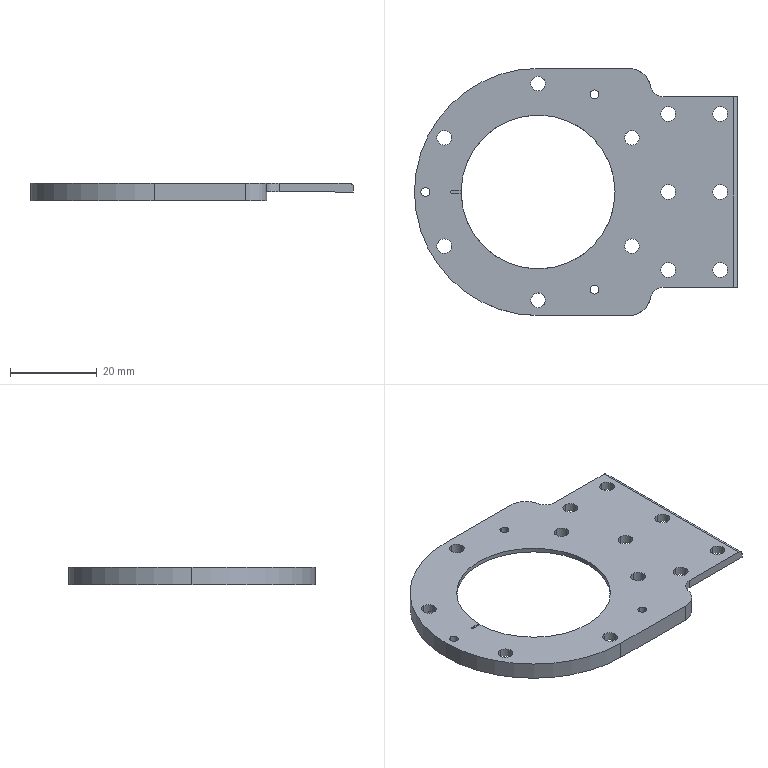NC program | NX | posted with a generic post | part box 74.5 x 57 x 4 mm
Lines 1 to 1524 of 3557:
N10 G17 G21 G94 G90
(FLOOR_WALL , TOOL : D80)
N12 T19 M6
N14 G54
N16 G17 G0 G90 X-82.25 Y0. S5000 M3
N18 G43 Z30. H19
N20 Z3.
N22 G94 G1 Z0. F1200.
N24 X-79.25
N26 X79.25
N28 X82.25
N30 Z3.
N32 G0 Z30.
N34 M5
(SPOT_DRILLING , TOOL : D6A45)
N36 T01 M6
N38 G54
N40 G17 G0 G90 X-8.75 Y-25. S9500 M3
N42 G43 Z30. H1
N44 G94 G82 G98 Z-1. F250. P200 R3.
N46 X4.25 Y-22.517
N48 X12.901 Y-12.5
N50 X21.25 Y-18.
N52 X33.25
N54 Y0.
N56 X21.25
N58 X33.25 Y18.
N60 X21.25
N62 X12.901 Y12.5
N64 X4.25 Y22.517
N66 X-8.75 Y25.
N68 X-30.401 Y12.5
N70 X-34.75 Y0.
N72 X-30.401 Y-12.5
N74 G80
N76 G0 X-30.401 Y-12.5 Z30.
N78 M5
(SPOT_DRILLING_COPY , TOOL : 2.1ZT)
N80 T17 M6
N82 G54
N84 G17 G0 G90 X4.25 Y22.517 S2500 M3
N86 G43 Z30. H17
N88 G94 G83 G98 Z-4.601 F120. Q2. R3.
N90 Y-22.517
N92 X-34.75 Y0.
N94 G80
N96 G0 X-34.75 Y0. Z30.
N98 M5
(SPOT_DRILLING_COPY_COPY , TOOL : 3.4ZT)
N100 T07 M6
N102 G54
N104 G17 G0 G90 X-8.75 Y-25. S2500 M3
N106 G43 Z30. H7
N108 G94 G83 G98 Z-5.021 F120. Q2. R3.
N110 X-30.401 Y-12.5
N112 Y12.5
N114 X-8.75 Y25.
N116 X12.901 Y12.5
N118 X21.25 Y18. Z-3.021
N120 X33.25
N122 Y0.
N124 X21.25
N126 X12.901 Y-12.5 Z-5.021
N128 X21.25 Y-18. Z-3.021
N130 X33.25
N132 G80
N134 G0 X33.25 Y-18. Z30.
N136 M5
(ZLEVEL_PROFILE , TOOL : D10)
N138 T15 M6
N140 G54
N142 G17 G0 G90 X3.196 Y33.6 S9500 M3
N144 G43 Z30. H15
N146 Z1.5
N148 G94 G1 X13.029 Z0.985 F1000.
N150 X15.122 Y33.214 Z0.873
N152 X17.088 Y32.4 Z0.762
N154 X18.841 Y31.193 Z0.65
N156 X20.303 Y29.646 Z0.539
N158 X21.409 Y27.828 Z0.427
N160 X21.687 Y27.1 Z0.386
N162 X37.239 Z-0.429
N164 X37.793 Z-0.458
N166 X39.138 Y26.766 Z-0.531
N168 X40.344 Y26.084 Z-0.603
N170 X41.323 Y25.105 Z-0.676
N172 X42.005 Y23.899 Z-0.748
N174 X42.34 Y22.554 Z-0.821
N176 Y22. Z-0.85
N178 Y-22. F3500.
N180 G2 X37.239 Y-27.1 R5.1
N182 G1 X21.687
N184 G2 X12.25 Y-33.6 R10.1
N186 G1 X-8.75
N188 G2 X-42.35 Y0. R33.6
N190 X-8.75 Y33.6 R33.6
N192 G1 X12.25
N194 G2 X21.687 Y27.1 R10.1
N196 G1 X37.239
N198 G2 X42.34 Y22. R5.1
N200 G1 X42.342 Y17.6 Z-0.864
N202 X42.343 Y13.2 Z-0.878
N204 X42.345 Y8.8 Z-0.893
N206 X42.346 Y4.4 Z-0.907
N208 X42.347 Y0. Z-0.921
N210 X42.348 Y-4.4 Z-0.935
N212 X42.349 Y-8.8 Z-0.95
N214 Y-13.2 Z-0.964
N216 X42.35 Y-17.6 Z-0.978
N218 Y-22. Z-0.992
N220 X42.325 Y-22.501 Z-0.994
N222 X42.251 Y-22.997 Z-0.995
N224 X42.129 Y-23.483 Z-0.997
N226 X41.96 Y-23.955 Z-0.999
N228 X41.745 Y-24.409 Z-1.
N230 X41.487 Y-24.838 Z-1.002
N232 X41.188 Y-25.241 Z-1.004
N234 X40.851 Y-25.612 Z-1.005
N236 X40.479 Y-25.948 Z-1.007
N238 X40.076 Y-26.246 Z-1.008
N240 X39.646 Y-26.502 Z-1.01
N242 X39.192 Y-26.716 Z-1.012
N244 X38.72 Y-26.883 Z-1.013
N246 X38.234 Y-27.004 Z-1.015
N248 X37.745 Y-27.076 Z-1.016
N250 X37.25 Y-27.1 Z-1.018
N252 X21.687 Z-1.068
N254 X21.385 Y-27.809 Z-1.071
N256 X21.039 Y-28.477 Z-1.073
N258 X20.639 Y-29.125 Z-1.076
N260 X20.191 Y-29.741 Z-1.078
N262 X19.699 Y-30.321 Z-1.081
N264 X19.164 Y-30.863 Z-1.083
N266 X18.59 Y-31.363 Z-1.086
N268 X17.979 Y-31.818 Z-1.088
N270 X17.336 Y-32.226 Z-1.09
N272 X16.665 Y-32.584 Z-1.093
N274 X15.968 Y-32.891 Z-1.095
N276 X15.25 Y-33.144 Z-1.098
N278 X14.515 Y-33.343 Z-1.1
N280 X13.767 Y-33.485 Z-1.103
N282 X13.011 Y-33.571 Z-1.105
N284 X12.25 Y-33.6 Z-1.108
N286 X-8.75 Z-1.176
N288 X-10.139 Y-33.571 Z-1.18
N290 X-11.526 Y-33.485 Z-1.185
N292 X-12.908 Y-33.342 Z-1.189
N294 X-14.283 Y-33.141 Z-1.194
N296 X-15.648 Y-32.884 Z-1.198
N298 X-17.002 Y-32.571 Z-1.202
N300 X-18.342 Y-32.202 Z-1.207
N302 X-19.665 Y-31.778 Z-1.211
N304 X-20.969 Y-31.299 Z-1.216
N306 X-22.253 Y-30.767 Z-1.22
N308 X-23.513 Y-30.183 Z-1.225
N310 X-24.749 Y-29.547 Z-1.229
N312 X-25.956 Y-28.86 Z-1.234
N314 X-27.135 Y-28.124 Z-1.238
N316 X-28.282 Y-27.34 Z-1.243
N318 X-29.396 Y-26.509 Z-1.247
N320 X-30.474 Y-25.633 Z-1.252
N322 X-31.515 Y-24.713 Z-1.256
N324 X-32.517 Y-23.75 Z-1.261
N326 X-33.479 Y-22.747 Z-1.265
N328 X-34.398 Y-21.705 Z-1.27
N330 X-35.274 Y-20.627 Z-1.274
N332 X-36.104 Y-19.512 Z-1.279
N334 X-36.887 Y-18.365 Z-1.283
N336 X-37.622 Y-17.186 Z-1.288
N338 X-38.308 Y-15.977 Z-1.292
N340 X-38.943 Y-14.742 Z-1.297
N342 X-39.527 Y-13.481 Z-1.301
N344 X-40.058 Y-12.197 Z-1.306
N346 X-40.536 Y-10.892 Z-1.31
N348 X-40.959 Y-9.568 Z-1.315
N350 X-41.327 Y-8.229 Z-1.319
N352 X-41.639 Y-6.875 Z-1.324
N354 X-41.895 Y-5.509 Z-1.328
N356 X-42.095 Y-4.134 Z-1.333
N358 X-42.237 Y-2.752 Z-1.337
N360 X-42.322 Y-1.365 Z-1.342
N362 X-42.35 Y0.024 Z-1.346
N364 X-42.32 Y1.412 Z-1.351
N366 X-42.233 Y2.797 Z-1.355
N368 X-42.089 Y4.178 Z-1.36
N370 X-41.888 Y5.552 Z-1.364
N372 X-41.631 Y6.916 Z-1.369
N374 X-41.317 Y8.268 Z-1.373
N376 X-40.948 Y9.606 Z-1.378
N378 X-40.523 Y10.928 Z-1.382
N380 X-40.045 Y12.231 Z-1.387
N382 X-39.513 Y13.513 Z-1.391
N384 X-38.928 Y14.772 Z-1.396
N386 X-38.292 Y16.006 Z-1.4
N388 X-37.606 Y17.213 Z-1.404
N390 X-36.87 Y18.39 Z-1.409
N392 X-36.087 Y19.536 Z-1.413
N394 X-35.257 Y20.649 Z-1.418
N396 X-34.381 Y21.726 Z-1.422
N398 X-33.462 Y22.766 Z-1.427
N400 X-32.5 Y23.767 Z-1.431
N402 X-31.498 Y24.728 Z-1.436
N404 X-30.457 Y25.647 Z-1.44
N406 X-29.38 Y26.521 Z-1.445
N408 X-28.266 Y27.351 Z-1.449
N410 X-27.12 Y28.134 Z-1.454
N412 X-25.942 Y28.868 Z-1.458
N414 X-24.735 Y29.554 Z-1.463
N416 X-23.501 Y30.189 Z-1.467
N418 X-22.241 Y30.773 Z-1.472
N420 X-20.959 Y31.304 Z-1.476
N422 X-19.655 Y31.781 Z-1.481
N424 X-18.333 Y32.204 Z-1.485
N426 X-16.995 Y32.573 Z-1.49
N428 X-15.642 Y32.886 Z-1.494
N430 X-14.278 Y33.142 Z-1.499
N432 X-12.904 Y33.342 Z-1.503
N434 X-11.523 Y33.485 Z-1.508
N436 X-10.138 Y33.571 Z-1.512
N438 X-8.75 Y33.6 Z-1.517
N440 X12.25 Z-1.585
N442 X13.011 Y33.571 Z-1.587
N444 X13.767 Y33.485 Z-1.589
N446 X14.515 Y33.343 Z-1.592
N448 X15.25 Y33.144 Z-1.594
N450 X15.968 Y32.891 Z-1.597
N452 X16.665 Y32.584 Z-1.599
N454 X17.336 Y32.226 Z-1.602
N456 X17.979 Y31.818 Z-1.604
N458 X18.59 Y31.363 Z-1.607
N460 X19.164 Y30.863 Z-1.609
N462 X19.699 Y30.321 Z-1.612
N464 X20.191 Y29.741 Z-1.614
N466 X20.639 Y29.125 Z-1.616
N468 X21.039 Y28.477 Z-1.619
N470 X21.385 Y27.809 Z-1.621
N472 X21.687 Y27.1 Z-1.624
N474 X37.25 Z-1.674
N476 X37.745 Y27.076 Z-1.676
N478 X38.234 Y27.004 Z-1.677
N480 X38.72 Y26.883 Z-1.679
N482 X39.192 Y26.716 Z-1.681
N484 X39.646 Y26.502 Z-1.682
N486 X40.076 Y26.246 Z-1.684
N488 X40.479 Y25.948 Z-1.685
N490 X40.851 Y25.612 Z-1.687
N492 X41.188 Y25.241 Z-1.689
N494 X41.487 Y24.838 Z-1.69
N496 X41.745 Y24.409 Z-1.692
N498 X41.96 Y23.956 Z-1.694
N500 X42.129 Y23.483 Z-1.695
N502 X42.252 Y22.997 Z-1.697
N504 X42.325 Y22.501 Z-1.698
N506 X42.35 Y22. Z-1.7
N508 Y-22. Z-1.842
N510 X42.325 Y-22.5 Z-1.844
N512 X42.252 Y-22.995 Z-1.845
N514 X42.13 Y-23.48 Z-1.847
N516 X41.962 Y-23.952 Z-1.849
N518 X41.748 Y-24.404 Z-1.85
N520 X41.49 Y-24.833 Z-1.852
N522 X41.192 Y-25.235 Z-1.854
N524 X40.856 Y-25.606 Z-1.855
N526 X40.485 Y-25.942 Z-1.857
N528 X40.083 Y-26.24 Z-1.858
N530 X39.654 Y-26.498 Z-1.86
N532 X39.202 Y-26.712 Z-1.862
N534 X38.73 Y-26.88 Z-1.863
N536 X38.245 Y-27.002 Z-1.865
N538 X37.75 Y-27.075 Z-1.866
N540 X37.25 Y-27.1 Z-1.868
N542 X21.687 Z-1.918
N544 X21.385 Y-27.809 Z-1.921
N546 X21.039 Y-28.477 Z-1.923
N548 X20.639 Y-29.125 Z-1.926
N550 X20.191 Y-29.741 Z-1.928
N552 X19.699 Y-30.321 Z-1.931
N554 X19.164 Y-30.863 Z-1.933
N556 X18.59 Y-31.363 Z-1.936
N558 X17.979 Y-31.818 Z-1.938
N560 X17.336 Y-32.226 Z-1.94
N562 X16.665 Y-32.584 Z-1.943
N564 X15.968 Y-32.891 Z-1.945
N566 X15.25 Y-33.144 Z-1.948
N568 X14.515 Y-33.343 Z-1.95
N570 X13.767 Y-33.485 Z-1.953
N572 X13.011 Y-33.571 Z-1.955
N574 X12.25 Y-33.6 Z-1.958
N576 X-8.75 Z-2.026
N578 X-10.139 Y-33.571 Z-2.03
N580 X-11.526 Y-33.485 Z-2.035
N582 X-12.908 Y-33.342 Z-2.039
N584 X-14.283 Y-33.141 Z-2.044
N586 X-15.648 Y-32.884 Z-2.048
N588 X-17.002 Y-32.571 Z-2.053
N590 X-18.342 Y-32.202 Z-2.057
N592 X-19.665 Y-31.778 Z-2.061
N594 X-20.969 Y-31.299 Z-2.066
N596 X-22.253 Y-30.767 Z-2.07
N598 X-23.513 Y-30.183 Z-2.075
N600 X-24.749 Y-29.547 Z-2.079
N602 X-25.956 Y-28.86 Z-2.084
N604 X-27.135 Y-28.124 Z-2.088
N606 X-28.282 Y-27.34 Z-2.093
N608 X-29.396 Y-26.509 Z-2.097
N610 X-30.474 Y-25.633 Z-2.102
N612 X-31.515 Y-24.713 Z-2.106
N614 X-32.517 Y-23.75 Z-2.111
N616 X-33.479 Y-22.747 Z-2.115
N618 X-34.398 Y-21.705 Z-2.12
N620 X-35.274 Y-20.627 Z-2.124
N622 X-36.104 Y-19.512 Z-2.129
N624 X-36.887 Y-18.365 Z-2.133
N626 X-37.622 Y-17.186 Z-2.138
N628 X-38.308 Y-15.977 Z-2.142
N630 X-38.943 Y-14.742 Z-2.147
N632 X-39.527 Y-13.481 Z-2.151
N634 X-40.058 Y-12.197 Z-2.156
N636 X-40.536 Y-10.892 Z-2.16
N638 X-40.959 Y-9.568 Z-2.165
N640 X-41.327 Y-8.229 Z-2.169
N642 X-41.639 Y-6.875 Z-2.174
N644 X-41.895 Y-5.509 Z-2.178
N646 X-42.095 Y-4.134 Z-2.183
N648 X-42.237 Y-2.752 Z-2.187
N650 X-42.322 Y-1.365 Z-2.192
N652 X-42.35 Y0.024 Z-2.196
N654 X-42.32 Y1.412 Z-2.201
N656 X-42.233 Y2.797 Z-2.205
N658 X-42.089 Y4.178 Z-2.21
N660 X-41.888 Y5.552 Z-2.214
N662 X-41.631 Y6.916 Z-2.219
N664 X-41.317 Y8.268 Z-2.223
N666 X-40.948 Y9.606 Z-2.228
N668 X-40.523 Y10.928 Z-2.232
N670 X-40.045 Y12.231 Z-2.237
N672 X-39.513 Y13.513 Z-2.241
N674 X-38.928 Y14.772 Z-2.246
N676 X-38.292 Y16.006 Z-2.25
N678 X-37.606 Y17.213 Z-2.254
N680 X-36.87 Y18.39 Z-2.259
N682 X-36.087 Y19.536 Z-2.263
N684 X-35.257 Y20.649 Z-2.268
N686 X-34.381 Y21.726 Z-2.272
N688 X-33.462 Y22.766 Z-2.277
N690 X-32.5 Y23.767 Z-2.281
N692 X-31.498 Y24.728 Z-2.286
N694 X-30.457 Y25.647 Z-2.29
N696 X-29.38 Y26.521 Z-2.295
N698 X-28.266 Y27.351 Z-2.299
N700 X-27.12 Y28.134 Z-2.304
N702 X-25.942 Y28.868 Z-2.308
N704 X-24.735 Y29.554 Z-2.313
N706 X-23.501 Y30.189 Z-2.317
N708 X-22.241 Y30.773 Z-2.322
N710 X-20.959 Y31.304 Z-2.326
N712 X-19.655 Y31.781 Z-2.331
N714 X-18.333 Y32.204 Z-2.335
N716 X-16.995 Y32.573 Z-2.34
N718 X-15.642 Y32.886 Z-2.344
N720 X-14.278 Y33.142 Z-2.349
N722 X-12.904 Y33.342 Z-2.353
N724 X-11.523 Y33.485 Z-2.358
N726 X-10.138 Y33.571 Z-2.362
N728 X-8.75 Y33.6 Z-2.367
N730 X12.25 Z-2.435
N732 X13.011 Y33.571 Z-2.437
N734 X13.767 Y33.485 Z-2.439
N736 X14.515 Y33.343 Z-2.442
N738 X15.25 Y33.144 Z-2.444
N740 X15.968 Y32.891 Z-2.447
N742 X16.665 Y32.584 Z-2.449
N744 X17.336 Y32.226 Z-2.452
N746 X17.979 Y31.818 Z-2.454
N748 X18.59 Y31.363 Z-2.457
N750 X19.164 Y30.863 Z-2.459
N752 X19.699 Y30.321 Z-2.462
N754 X20.191 Y29.741 Z-2.464
N756 X20.639 Y29.125 Z-2.466
N758 X21.039 Y28.477 Z-2.469
N760 X21.385 Y27.809 Z-2.471
N762 X21.687 Y27.1 Z-2.474
N764 X37.25 Z-2.524
N766 X37.75 Y27.075 Z-2.526
N768 X38.245 Y27.002 Z-2.527
N770 X38.73 Y26.88 Z-2.529
N772 X39.202 Y26.712 Z-2.531
N774 X39.654 Y26.498 Z-2.532
N776 X40.083 Y26.241 Z-2.534
N778 X40.485 Y25.942 Z-2.535
N780 X40.856 Y25.606 Z-2.537
N782 X41.192 Y25.235 Z-2.539
N784 X41.49 Y24.833 Z-2.54
N786 X41.748 Y24.404 Z-2.542
N788 X41.962 Y23.952 Z-2.544
N790 X42.13 Y23.48 Z-2.545
N792 X42.252 Y22.995 Z-2.547
N794 X42.325 Y22.5 Z-2.548
N796 X42.35 Y22. Z-2.55
N798 Y-22. Z-2.692
N800 X42.325 Y-22.5 Z-2.694
N802 X42.252 Y-22.995 Z-2.695
N804 X42.13 Y-23.48 Z-2.697
N806 X41.962 Y-23.952 Z-2.699
N808 X41.748 Y-24.404 Z-2.7
N810 X41.49 Y-24.833 Z-2.702
N812 X41.192 Y-25.235 Z-2.704
N814 X40.856 Y-25.606 Z-2.705
N816 X40.485 Y-25.942 Z-2.707
N818 X40.083 Y-26.24 Z-2.708
N820 X39.654 Y-26.498 Z-2.71
N822 X39.202 Y-26.712 Z-2.712
N824 X38.73 Y-26.88 Z-2.713
N826 X38.245 Y-27.002 Z-2.715
N828 X37.75 Y-27.075 Z-2.716
N830 X37.25 Y-27.1 Z-2.718
N832 X21.687 Z-2.768
N834 X21.385 Y-27.809 Z-2.771
N836 X21.039 Y-28.477 Z-2.773
N838 X20.639 Y-29.125 Z-2.776
N840 X20.191 Y-29.741 Z-2.778
N842 X19.699 Y-30.321 Z-2.781
N844 X19.164 Y-30.863 Z-2.783
N846 X18.59 Y-31.363 Z-2.786
N848 X17.979 Y-31.818 Z-2.788
N850 X17.336 Y-32.226 Z-2.79
N852 X16.665 Y-32.584 Z-2.793
N854 X15.968 Y-32.891 Z-2.795
N856 X15.25 Y-33.144 Z-2.798
N858 X14.515 Y-33.343 Z-2.8
N860 X13.767 Y-33.485 Z-2.803
N862 X13.011 Y-33.571 Z-2.805
N864 X12.25 Y-33.6 Z-2.808
N866 X-8.75 Z-2.876
N868 X-10.139 Y-33.571 Z-2.88
N870 X-11.526 Y-33.485 Z-2.885
N872 X-12.908 Y-33.342 Z-2.889
N874 X-14.283 Y-33.141 Z-2.894
N876 X-15.648 Y-32.884 Z-2.898
N878 X-17.002 Y-32.571 Z-2.903
N880 X-18.342 Y-32.202 Z-2.907
N882 X-19.665 Y-31.778 Z-2.911
N884 X-20.969 Y-31.299 Z-2.916
N886 X-22.253 Y-30.767 Z-2.92
N888 X-23.513 Y-30.183 Z-2.925
N890 X-24.749 Y-29.547 Z-2.929
N892 X-25.956 Y-28.86 Z-2.934
N894 X-27.135 Y-28.124 Z-2.938
N896 X-28.282 Y-27.34 Z-2.943
N898 X-29.396 Y-26.509 Z-2.947
N900 X-30.474 Y-25.633 Z-2.952
N902 X-31.515 Y-24.713 Z-2.956
N904 X-32.517 Y-23.75 Z-2.961
N906 X-33.479 Y-22.747 Z-2.965
N908 X-34.398 Y-21.705 Z-2.97
N910 X-35.274 Y-20.627 Z-2.974
N912 X-36.104 Y-19.512 Z-2.979
N914 X-36.887 Y-18.365 Z-2.983
N916 X-37.622 Y-17.186 Z-2.988
N918 X-38.308 Y-15.977 Z-2.992
N920 X-38.943 Y-14.742 Z-2.997
N922 X-39.527 Y-13.481 Z-3.001
N924 X-40.058 Y-12.197 Z-3.006
N926 X-40.536 Y-10.892 Z-3.01
N928 X-40.959 Y-9.568 Z-3.015
N930 X-41.327 Y-8.229 Z-3.019
N932 X-41.639 Y-6.875 Z-3.024
N934 X-41.895 Y-5.509 Z-3.028
N936 X-42.095 Y-4.134 Z-3.033
N938 X-42.237 Y-2.752 Z-3.037
N940 X-42.322 Y-1.365 Z-3.042
N942 X-42.35 Y0.024 Z-3.046
N944 X-42.32 Y1.412 Z-3.051
N946 X-42.233 Y2.797 Z-3.055
N948 X-42.089 Y4.178 Z-3.06
N950 X-41.888 Y5.552 Z-3.064
N952 X-41.631 Y6.916 Z-3.069
N954 X-41.317 Y8.268 Z-3.073
N956 X-40.948 Y9.606 Z-3.078
N958 X-40.523 Y10.928 Z-3.082
N960 X-40.045 Y12.231 Z-3.087
N962 X-39.513 Y13.513 Z-3.091
N964 X-38.928 Y14.772 Z-3.096
N966 X-38.292 Y16.006 Z-3.1
N968 X-37.606 Y17.213 Z-3.104
N970 X-36.87 Y18.39 Z-3.109
N972 X-36.087 Y19.536 Z-3.113
N974 X-35.257 Y20.649 Z-3.118
N976 X-34.381 Y21.726 Z-3.122
N978 X-33.462 Y22.766 Z-3.127
N980 X-32.5 Y23.767 Z-3.131
N982 X-31.498 Y24.728 Z-3.136
N984 X-30.457 Y25.647 Z-3.14
N986 X-29.38 Y26.521 Z-3.145
N988 X-28.266 Y27.351 Z-3.149
N990 X-27.12 Y28.134 Z-3.154
N992 X-25.942 Y28.868 Z-3.158
N994 X-24.735 Y29.554 Z-3.163
N996 X-23.501 Y30.189 Z-3.167
N998 X-22.241 Y30.773 Z-3.172
N1000 X-20.959 Y31.304 Z-3.176
N1002 X-19.655 Y31.781 Z-3.181
N1004 X-18.333 Y32.204 Z-3.185
N1006 X-16.995 Y32.573 Z-3.19
N1008 X-15.642 Y32.886 Z-3.194
N1010 X-14.278 Y33.142 Z-3.199
N1012 X-12.904 Y33.342 Z-3.203
N1014 X-11.523 Y33.485 Z-3.208
N1016 X-10.138 Y33.571 Z-3.212
N1018 X-8.75 Y33.6 Z-3.217
N1020 X12.25 Z-3.285
N1022 X13.011 Y33.571 Z-3.287
N1024 X13.767 Y33.485 Z-3.289
N1026 X14.515 Y33.343 Z-3.292
N1028 X15.25 Y33.144 Z-3.294
N1030 X15.968 Y32.891 Z-3.297
N1032 X16.665 Y32.584 Z-3.299
N1034 X17.336 Y32.226 Z-3.302
N1036 X17.979 Y31.818 Z-3.304
N1038 X18.59 Y31.363 Z-3.307
N1040 X19.164 Y30.863 Z-3.309
N1042 X19.699 Y30.321 Z-3.312
N1044 X20.191 Y29.741 Z-3.314
N1046 X20.639 Y29.125 Z-3.316
N1048 X21.039 Y28.477 Z-3.319
N1050 X21.385 Y27.809 Z-3.321
N1052 X21.687 Y27.1 Z-3.324
N1054 X37.25 Z-3.374
N1056 X37.75 Y27.075 Z-3.376
N1058 X38.245 Y27.002 Z-3.377
N1060 X38.73 Y26.88 Z-3.379
N1062 X39.202 Y26.712 Z-3.381
N1064 X39.654 Y26.498 Z-3.382
N1066 X40.083 Y26.241 Z-3.384
N1068 X40.485 Y25.942 Z-3.385
N1070 X40.856 Y25.606 Z-3.387
N1072 X41.192 Y25.235 Z-3.389
N1074 X41.49 Y24.833 Z-3.39
N1076 X41.748 Y24.404 Z-3.392
N1078 X41.962 Y23.952 Z-3.394
N1080 X42.13 Y23.48 Z-3.395
N1082 X42.252 Y22.995 Z-3.397
N1084 X42.325 Y22.5 Z-3.398
N1086 X42.35 Y22. Z-3.4
N1088 Y-22.
N1090 G2 X37.25 Y-27.1 R5.1
N1092 G1 X21.687
N1094 G2 X12.25 Y-33.6 R10.1
N1096 G1 X-8.75
N1098 G2 X-42.35 Y0. R33.6
N1100 X-8.75 Y33.6 R33.6
N1102 G1 X12.25
N1104 G2 X21.687 Y27.1 R10.1
N1106 G1 X37.25
N1108 G2 X42.35 Y22. R5.1
N1110 G1 Z-1.9
N1112 G0 Z30.
(PLANAR_MILL_3 , TOOL : D10)
N1114 X-14.863 Y-0.634
N1116 Z1.5
N1118 G1 X-14.784 Y-1.24 Z1.468 F1000.
N1120 X-14.54 Y-2.103 Z1.421
N1122 X-14.173 Y-2.921 Z1.374
N1124 X-13.692 Y-3.677 Z1.327
N1126 X-13.106 Y-4.356 Z1.28
N1128 X-12.427 Y-4.942 Z1.233
N1130 X-11.671 Y-5.423 Z1.186
N1132 X-10.853 Y-5.79 Z1.139
N1134 X-9.99 Y-6.034 Z1.092
N1136 X-9.101 Y-6.15 Z1.045
N1138 X-8.399 Z1.008
N1140 X-7.51 Y-6.034 Z0.961
N1142 X-6.647 Y-5.79 Z0.914
N1144 X-5.829 Y-5.423 Z0.867
N1146 X-5.073 Y-4.942 Z0.82
N1148 X-4.394 Y-4.356 Z0.773
N1150 X-3.808 Y-3.677 Z0.726
N1152 X-3.327 Y-2.921 Z0.679
N1154 X-2.96 Y-2.103 Z0.632
N1156 X-2.716 Y-1.24 Z0.585
N1158 X-2.6 Y-0.351 Z0.538
N1160 Y0.351 Z0.502
N1162 X-2.716 Y1.24 Z0.455
N1164 X-2.96 Y2.103 Z0.408
N1166 X-3.327 Y2.921 Z0.361
N1168 X-3.808 Y3.677 Z0.314
N1170 X-4.394 Y4.356 Z0.267
N1172 X-5.073 Y4.942 Z0.22
N1174 X-5.829 Y5.423 Z0.173
N1176 X-6.647 Y5.79 Z0.126
N1178 X-7.51 Y6.034 Z0.079
N1180 X-8.399 Y6.15 Z0.032
N1182 X-9.101 Z-0.005
N1184 X-9.99 Y6.034 Z-0.052
N1186 X-10.853 Y5.79 Z-0.099
N1188 X-11.671 Y5.423 Z-0.146
N1190 X-12.427 Y4.942 Z-0.193
N1192 X-13.106 Y4.356 Z-0.24
N1194 X-13.692 Y3.677 Z-0.287
N1196 X-14.173 Y2.921 Z-0.334
N1198 X-14.54 Y2.103 Z-0.381
N1200 X-14.784 Y1.24 Z-0.428
N1202 X-14.9 Y0.351 Z-0.475
N1204 Y-0.351 Z-0.512
N1206 X-14.784 Y-1.24 Z-0.559
N1208 X-14.54 Y-2.103 Z-0.606
N1210 X-14.173 Y-2.921 Z-0.653
N1212 X-13.692 Y-3.677 Z-0.7
N1214 X-13.106 Y-4.356 Z-0.747
N1216 X-12.427 Y-4.942 Z-0.794
N1218 X-11.671 Y-5.423 Z-0.841
N1220 X-10.853 Y-5.79 Z-0.888
N1222 X-9.99 Y-6.034 Z-0.935
N1224 X-9.101 Y-6.15 Z-0.982
N1226 X-8.75 Z-1.
N1228 Y-1.65
N1230 G3 X-7.1 Y0. R1.65 F3500.
N1232 X-8.75 Y-1.65 R-1.65
N1234 G1 Y-6.15
N1236 G3 X-2.6 Y0. R6.15
N1238 X-8.75 Y-6.15 R-6.15
N1240 G1 Y-12.65
N1242 G3 X3.9 Y0. R12.65
N1244 X-8.75 Y-12.65 R-12.65
N1246 G1 Z0.5
N1248 G0 X-14.863 Y-0.634
N1250 G1 X-14.784 Y-1.24 Z0.468 F1000.
N1252 X-14.54 Y-2.103 Z0.421
N1254 X-14.173 Y-2.921 Z0.374
N1256 X-13.692 Y-3.677 Z0.327
N1258 X-13.106 Y-4.356 Z0.28
N1260 X-12.427 Y-4.942 Z0.233
N1262 X-11.671 Y-5.423 Z0.186
N1264 X-10.853 Y-5.79 Z0.139
N1266 X-9.99 Y-6.034 Z0.092
N1268 X-9.101 Y-6.15 Z0.045
N1270 X-8.399 Z0.008
N1272 X-7.51 Y-6.034 Z-0.039
N1274 X-6.647 Y-5.79 Z-0.086
N1276 X-5.829 Y-5.423 Z-0.133
N1278 X-5.073 Y-4.942 Z-0.18
N1280 X-4.394 Y-4.356 Z-0.227
N1282 X-3.808 Y-3.677 Z-0.274
N1284 X-3.327 Y-2.921 Z-0.321
N1286 X-2.96 Y-2.103 Z-0.368
N1288 X-2.716 Y-1.24 Z-0.415
N1290 X-2.6 Y-0.351 Z-0.462
N1292 Y0.351 Z-0.498
N1294 X-2.716 Y1.24 Z-0.545
N1296 X-2.96 Y2.103 Z-0.592
N1298 X-3.327 Y2.921 Z-0.639
N1300 X-3.808 Y3.677 Z-0.686
N1302 X-4.394 Y4.356 Z-0.733
N1304 X-5.073 Y4.942 Z-0.78
N1306 X-5.829 Y5.423 Z-0.827
N1308 X-6.647 Y5.79 Z-0.874
N1310 X-7.51 Y6.034 Z-0.921
N1312 X-8.399 Y6.15 Z-0.968
N1314 X-9.101 Z-1.005
N1316 X-9.99 Y6.034 Z-1.052
N1318 X-10.853 Y5.79 Z-1.099
N1320 X-11.671 Y5.423 Z-1.146
N1322 X-12.427 Y4.942 Z-1.193
N1324 X-13.106 Y4.356 Z-1.24
N1326 X-13.692 Y3.677 Z-1.287
N1328 X-14.173 Y2.921 Z-1.334
N1330 X-14.54 Y2.103 Z-1.381
N1332 X-14.784 Y1.24 Z-1.428
N1334 X-14.9 Y0.351 Z-1.475
N1336 Y-0.351 Z-1.512
N1338 X-14.784 Y-1.24 Z-1.559
N1340 X-14.54 Y-2.103 Z-1.606
N1342 X-14.173 Y-2.921 Z-1.653
N1344 X-13.692 Y-3.677 Z-1.7
N1346 X-13.106 Y-4.356 Z-1.747
N1348 X-12.427 Y-4.942 Z-1.794
N1350 X-11.671 Y-5.423 Z-1.841
N1352 X-10.853 Y-5.79 Z-1.888
N1354 X-9.99 Y-6.034 Z-1.935
N1356 X-9.101 Y-6.15 Z-1.982
N1358 X-8.75 Z-2.
N1360 Y-1.65
N1362 G3 X-7.1 Y0. R1.65 F3500.
N1364 X-8.75 Y-1.65 R-1.65
N1366 G1 Y-6.15
N1368 G3 X-2.6 Y0. R6.15
N1370 X-8.75 Y-6.15 R-6.15
N1372 G1 Y-12.65
N1374 G3 X3.9 Y0. R12.65
N1376 X-8.75 Y-12.65 R-12.65
N1378 G1 Z-0.5
N1380 G0 X-14.863 Y-0.634
N1382 G1 X-14.784 Y-1.24 Z-0.532 F1000.
N1384 X-14.54 Y-2.103 Z-0.579
N1386 X-14.173 Y-2.921 Z-0.626
N1388 X-13.692 Y-3.677 Z-0.673
N1390 X-13.106 Y-4.356 Z-0.72
N1392 X-12.427 Y-4.942 Z-0.767
N1394 X-11.671 Y-5.423 Z-0.814
N1396 X-10.853 Y-5.79 Z-0.861
N1398 X-9.99 Y-6.034 Z-0.908
N1400 X-9.101 Y-6.15 Z-0.955
N1402 X-8.399 Z-0.992
N1404 X-7.51 Y-6.034 Z-1.039
N1406 X-6.647 Y-5.79 Z-1.086
N1408 X-5.829 Y-5.423 Z-1.133
N1410 X-5.073 Y-4.942 Z-1.18
N1412 X-4.394 Y-4.356 Z-1.227
N1414 X-3.808 Y-3.677 Z-1.274
N1416 X-3.327 Y-2.921 Z-1.321
N1418 X-2.96 Y-2.103 Z-1.368
N1420 X-2.716 Y-1.24 Z-1.415
N1422 X-2.6 Y-0.351 Z-1.462
N1424 Y0.351 Z-1.498
N1426 X-2.716 Y1.24 Z-1.545
N1428 X-2.96 Y2.103 Z-1.592
N1430 X-3.327 Y2.921 Z-1.639
N1432 X-3.808 Y3.677 Z-1.686
N1434 X-4.394 Y4.356 Z-1.733
N1436 X-5.073 Y4.942 Z-1.78
N1438 X-5.829 Y5.423 Z-1.827
N1440 X-6.647 Y5.79 Z-1.874
N1442 X-7.51 Y6.034 Z-1.921
N1444 X-8.399 Y6.15 Z-1.968
N1446 X-9.101 Z-2.005
N1448 X-9.99 Y6.034 Z-2.052
N1450 X-10.853 Y5.79 Z-2.099
N1452 X-11.671 Y5.423 Z-2.146
N1454 X-12.427 Y4.942 Z-2.193
N1456 X-13.106 Y4.356 Z-2.24
N1458 X-13.692 Y3.677 Z-2.287
N1460 X-14.173 Y2.921 Z-2.334
N1462 X-14.54 Y2.103 Z-2.381
N1464 X-14.784 Y1.24 Z-2.428
N1466 X-14.9 Y0.351 Z-2.475
N1468 Y-0.351 Z-2.512
N1470 X-14.784 Y-1.24 Z-2.559
N1472 X-14.54 Y-2.103 Z-2.606
N1474 X-14.173 Y-2.921 Z-2.653
N1476 X-13.692 Y-3.677 Z-2.7
N1478 X-13.106 Y-4.356 Z-2.747
N1480 X-12.427 Y-4.942 Z-2.794
N1482 X-11.671 Y-5.423 Z-2.841
N1484 X-10.853 Y-5.79 Z-2.888
N1486 X-9.99 Y-6.034 Z-2.935
N1488 X-9.101 Y-6.15 Z-2.982
N1490 X-8.75 Z-3.
N1492 Y-1.65
N1494 G3 X-7.1 Y0. R1.65 F3500.
N1496 X-8.75 Y-1.65 R-1.65
N1498 G1 Y-6.15
N1500 G3 X-2.6 Y0. R6.15
N1502 X-8.75 Y-6.15 R-6.15
N1504 G1 Y-12.65
N1506 G3 X3.9 Y0. R12.65
N1508 X-8.75 Y-12.65 R-12.65
N1510 G1 Z-1.5
N1512 G0 X-14.863 Y-0.634
N1514 G1 X-14.784 Y-1.24 Z-1.532 F1000.
N1516 X-14.54 Y-2.103 Z-1.579
N1518 X-14.173 Y-2.921 Z-1.626
N1520 X-13.692 Y-3.677 Z-1.673
N1522 X-13.106 Y-4.356 Z-1.72
N1524 X-12.427 Y-4.942 Z-1.767
N1526 X-11.671 Y-5.423 Z-1.814
N1528 X-10.853 Y-5.79 Z-1.861
N1530 X-9.99 Y-6.034 Z-1.908
N1532 X-9.101 Y-6.15 Z-1.955
N1534 X-8.399 Z-1.992
N1536 X-7.51 Y-6.034 Z-2.039
N1538 X-6.647 Y-5.79 Z-2.086
N1540 X-5.829 Y-5.423 Z-2.133
N1542 X-5.073 Y-4.942 Z-2.18
N1544 X-4.394 Y-4.356 Z-2.227
N1546 X-3.808 Y-3.677 Z-2.274
N1548 X-3.327 Y-2.921 Z-2.321
N1550 X-2.96 Y-2.103 Z-2.368
N1552 X-2.716 Y-1.24 Z-2.415
N1554 X-2.6 Y-0.351 Z-2.462
N1556 Y0.351 Z-2.498
N1558 X-2.716 Y1.24 Z-2.545
N1560 X-2.96 Y2.103 Z-2.592
N1562 X-3.327 Y2.921 Z-2.639
N1564 X-3.808 Y3.677 Z-2.686
N1566 X-4.394 Y4.356 Z-2.733
N1568 X-5.073 Y4.942 Z-2.78
N1570 X-5.829 Y5.423 Z-2.827
N1572 X-6.647 Y5.79 Z-2.874
N1574 X-7.51 Y6.034 Z-2.921
N1576 X-8.399 Y6.15 Z-2.968
N1578 X-9.101 Z-3.005
N1580 X-9.99 Y6.034 Z-3.052
N1582 X-10.853 Y5.79 Z-3.099
N1584 X-11.671 Y5.423 Z-3.146
N1586 X-12.427 Y4.942 Z-3.193
N1588 X-13.106 Y4.356 Z-3.24
N1590 X-13.692 Y3.677 Z-3.287
N1592 X-14.173 Y2.921 Z-3.334
N1594 X-14.54 Y2.103 Z-3.381
N1596 X-14.784 Y1.24 Z-3.428
N1598 X-14.9 Y0.351 Z-3.475
N1600 Y-0.351 Z-3.512
N1602 X-14.784 Y-1.24 Z-3.559
N1604 X-14.54 Y-2.103 Z-3.606
N1606 X-14.173 Y-2.921 Z-3.653
N1608 X-13.692 Y-3.677 Z-3.7
N1610 X-13.106 Y-4.356 Z-3.747
N1612 X-12.427 Y-4.942 Z-3.794
N1614 X-11.671 Y-5.423 Z-3.841
N1616 X-10.853 Y-5.79 Z-3.888
N1618 X-9.99 Y-6.034 Z-3.935
N1620 X-9.101 Y-6.15 Z-3.982
N1622 X-8.75 Z-4.
N1624 Y-1.65
N1626 G3 X-7.1 Y0. R1.65 F3500.
N1628 X-8.75 Y-1.65 R-1.65
N1630 G1 Y-6.15
N1632 G3 X-2.6 Y0. R6.15
N1634 X-8.75 Y-6.15 R-6.15
N1636 G1 Y-12.65
N1638 G3 X3.9 Y0. R12.65
N1640 X-8.75 Y-12.65 R-12.65
N1642 G1 Z-2.5
N1644 G0 Z30.
N1646 M5
(ZLEVEL_PROFILE_COPY_1 , TOOL : D3)
N1648 T16 M6
N1650 G54
N1652 G17 G0 G90 X18.613 Y26.651 S9500 M3
N1654 G43 Z30. H16
N1656 Z1.214
N1658 G94 G1 Z-0.286 F1000.
N1660 X18.307 Y26.257
N1662 G3 X18.267 Y25.959 R0.3
N1664 G2 X18.635 Y24.719 R6.5 F1200.
N1666 G3 X20.108 Y23.5 R1.5
N1668 G1 X21.743
N1670 G3 X22.003 Y23.65 R0.3
N1672 G1 X22.262 Y24.1
N1674 Z1.214
N1676 G0 X18.613 Y26.651 Z0.929
N1678 G1 Z-0.571 F1000.
N1680 X18.307 Y26.257
N1682 G3 X18.267 Y25.959 R0.3
N1684 G2 X18.635 Y24.719 R6.5 F1200.
N1686 G3 X20.108 Y23.5 R1.5
N1688 G1 X21.743
N1690 G3 X22.003 Y23.65 R0.3
N1692 G1 X22.262 Y24.1
N1694 Z0.929
N1696 G0 X18.613 Y26.651 Z0.643
N1698 G1 Z-0.857 F1000.
N1700 X18.307 Y26.257
N1702 G3 X18.267 Y25.959 R0.3
N1704 G2 X18.635 Y24.719 R6.5 F1200.
N1706 G3 X20.108 Y23.5 R1.5
N1708 G1 X21.743
N1710 G3 X22.003 Y23.65 R0.3
N1712 G1 X22.262 Y24.1
N1714 Z0.643
N1716 G0 X18.613 Y26.651 Z0.357
N1718 G1 Z-1.143 F1000.
N1720 X18.307 Y26.257
N1722 G3 X18.267 Y25.959 R0.3
N1724 G2 X18.635 Y24.719 R6.5 F1200.
N1726 G3 X20.108 Y23.5 R1.5
N1728 G1 X21.743
N1730 G3 X22.003 Y23.65 R0.3
N1732 G1 X22.262 Y24.1
N1734 Z0.357
N1736 G0 X18.613 Y26.651 Z0.071
N1738 G1 Z-1.429 F1000.
N1740 X18.307 Y26.257
N1742 G3 X18.267 Y25.959 R0.3
N1744 G2 X18.635 Y24.719 R6.5 F1200.
N1746 G3 X20.108 Y23.5 R1.5
N1748 G1 X21.743
N1750 G3 X22.003 Y23.65 R0.3
N1752 G1 X22.262 Y24.1
N1754 Z0.071
N1756 G0 X18.613 Y26.651 Z-0.214
N1758 G1 Z-1.714 F1000.
N1760 X18.307 Y26.257
N1762 G3 X18.267 Y25.959 R0.3
N1764 G2 X18.635 Y24.719 R6.5 F1200.
N1766 G3 X20.108 Y23.5 R1.5
N1768 G1 X21.743
N1770 G3 X22.003 Y23.65 R0.3
N1772 G1 X22.262 Y24.1
N1774 Z-0.214
N1776 G0 X18.613 Y26.651 Z-0.5
N1778 G1 Z-2. F1000.
N1780 X18.307 Y26.257
N1782 G3 X18.267 Y25.959 R0.3
N1784 G2 X18.635 Y24.719 R6.5 F1200.
N1786 G3 X20.108 Y23.5 R1.5
N1788 G1 X21.743
N1790 G3 X22.003 Y23.65 R0.3
N1792 G1 X22.262 Y24.1
N1794 Z-0.5
N1796 G0 X18.613 Y26.651 Z-0.786
N1798 G1 Z-2.286 F1000.
N1800 X18.307 Y26.257
N1802 G3 X18.267 Y25.959 R0.3
N1804 G2 X18.635 Y24.719 R6.5 F1200.
N1806 G3 X20.108 Y23.5 R1.5
N1808 G1 X21.743
N1810 G3 X22.003 Y23.65 R0.3
N1812 G1 X22.262 Y24.1
N1814 Z-0.786
N1816 G0 X18.613 Y26.651 Z-1.071
N1818 G1 Z-2.571 F1000.
N1820 X18.307 Y26.257
N1822 G3 X18.267 Y25.959 R0.3
N1824 G2 X18.635 Y24.719 R6.5 F1200.
N1826 G3 X20.108 Y23.5 R1.5
N1828 G1 X21.743
N1830 G3 X22.003 Y23.65 R0.3
N1832 G1 X22.262 Y24.1
N1834 Z-1.071
N1836 G0 X18.613 Y26.651 Z-1.357
N1838 G1 Z-2.857 F1000.
N1840 X18.307 Y26.257
N1842 G3 X18.267 Y25.959 R0.3
N1844 G2 X18.635 Y24.719 R6.5 F1200.
N1846 G3 X20.108 Y23.5 R1.5
N1848 G1 X21.743
N1850 G3 X22.003 Y23.65 R0.3
N1852 G1 X22.262 Y24.1
N1854 Z-1.357
N1856 G0 X18.613 Y26.651 Z-1.643
N1858 G1 Z-3.143 F1000.
N1860 X18.307 Y26.257
N1862 G3 X18.267 Y25.959 R0.3
N1864 G2 X18.635 Y24.719 R6.5 F1200.
N1866 G3 X20.108 Y23.5 R1.5
N1868 G1 X21.743
N1870 G3 X22.003 Y23.65 R0.3
N1872 G1 X22.262 Y24.1
N1874 Z-1.643
N1876 G0 X18.613 Y26.651 Z-1.929
N1878 G1 Z-3.429 F1000.
N1880 X18.307 Y26.257
N1882 G3 X18.267 Y25.959 R0.3
N1884 G2 X18.635 Y24.719 R6.5 F1200.
N1886 G3 X20.108 Y23.5 R1.5
N1888 G1 X21.743
N1890 G3 X22.003 Y23.65 R0.3
N1892 G1 X22.262 Y24.1
N1894 Z-1.929
N1896 G0 X18.613 Y26.651 Z-2.214
N1898 G1 Z-3.714 F1000.
N1900 X18.307 Y26.257
N1902 G3 X18.267 Y25.959 R0.3
N1904 G2 X18.635 Y24.719 R6.5 F1200.
N1906 G3 X20.108 Y23.5 R1.5
N1908 G1 X21.743
N1910 G3 X22.003 Y23.65 R0.3
N1912 G1 X22.262 Y24.1
N1914 Z-2.214
N1916 G0 X18.613 Y26.651 Z-2.5
N1918 G1 Z-4. F1000.
N1920 X18.307 Y26.257
N1922 G3 X18.267 Y25.959 R0.3
N1924 G2 X18.635 Y24.719 R6.5 F1200.
N1926 G3 X20.108 Y23.5 R1.5
N1928 G1 X21.743
N1930 G3 X22.003 Y23.65 R0.3
N1932 G1 X22.262 Y24.1
N1934 Z-2.5
N1936 G0 Z30.
N1938 Y-24.1
N1940 Z1.214
N1942 G1 Z-0.286 F1000.
N1944 X22.002 Y-23.65
N1946 G3 X21.743 Y-23.5 R0.3
N1948 G1 X20.108 F1200.
N1950 G3 X18.635 Y-24.719 R1.5
N1952 G2 X18.267 Y-25.958 R6.5
N1954 G3 X18.308 Y-26.255 R0.3
N1956 G1 X18.614 Y-26.649
N1958 Z1.214
N1960 G0 X22.262 Y-24.1 Z0.929
N1962 G1 Z-0.571 F1000.
N1964 X22.002 Y-23.65
N1966 G3 X21.743 Y-23.5 R0.3
N1968 G1 X20.108 F1200.
N1970 G3 X18.635 Y-24.719 R1.5
N1972 G2 X18.267 Y-25.958 R6.5
N1974 G3 X18.308 Y-26.255 R0.3
N1976 G1 X18.614 Y-26.649
N1978 Z0.929
N1980 G0 X22.262 Y-24.1 Z0.643
N1982 G1 Z-0.857 F1000.
N1984 X22.002 Y-23.65
N1986 G3 X21.743 Y-23.5 R0.3
N1988 G1 X20.108 F1200.
N1990 G3 X18.635 Y-24.719 R1.5
N1992 G2 X18.267 Y-25.958 R6.5
N1994 G3 X18.308 Y-26.255 R0.3
N1996 G1 X18.614 Y-26.649
N1998 Z0.643
N2000 G0 X22.262 Y-24.1 Z0.357
N2002 G1 Z-1.143 F1000.
N2004 X22.002 Y-23.65
N2006 G3 X21.743 Y-23.5 R0.3
N2008 G1 X20.108 F1200.
N2010 G3 X18.635 Y-24.719 R1.5
N2012 G2 X18.267 Y-25.958 R6.5
N2014 G3 X18.308 Y-26.255 R0.3
N2016 G1 X18.614 Y-26.649
N2018 Z0.357
N2020 G0 X22.262 Y-24.1 Z0.071
N2022 G1 Z-1.429 F1000.
N2024 X22.002 Y-23.65
N2026 G3 X21.743 Y-23.5 R0.3
N2028 G1 X20.108 F1200.
N2030 G3 X18.635 Y-24.719 R1.5
N2032 G2 X18.267 Y-25.958 R6.5
N2034 G3 X18.308 Y-26.255 R0.3
N2036 G1 X18.614 Y-26.649
N2038 Z0.071
N2040 G0 X22.262 Y-24.1 Z-0.214
N2042 G1 Z-1.714 F1000.
N2044 X22.002 Y-23.65
N2046 G3 X21.743 Y-23.5 R0.3
N2048 G1 X20.108 F1200.
N2050 G3 X18.635 Y-24.719 R1.5
N2052 G2 X18.267 Y-25.958 R6.5
N2054 G3 X18.308 Y-26.255 R0.3
N2056 G1 X18.614 Y-26.649
N2058 Z-0.214
N2060 G0 X22.262 Y-24.1 Z-0.5
N2062 G1 Z-2. F1000.
N2064 X22.002 Y-23.65
N2066 G3 X21.743 Y-23.5 R0.3
N2068 G1 X20.108 F1200.
N2070 G3 X18.635 Y-24.719 R1.5
N2072 G2 X18.267 Y-25.958 R6.5
N2074 G3 X18.308 Y-26.255 R0.3
N2076 G1 X18.614 Y-26.649
N2078 Z-0.5
N2080 G0 X22.262 Y-24.1 Z-0.786
N2082 G1 Z-2.286 F1000.
N2084 X22.002 Y-23.65
N2086 G3 X21.743 Y-23.5 R0.3
N2088 G1 X20.108 F1200.
N2090 G3 X18.635 Y-24.719 R1.5
N2092 G2 X18.267 Y-25.958 R6.5
N2094 G3 X18.308 Y-26.255 R0.3
N2096 G1 X18.614 Y-26.649
N2098 Z-0.786
N2100 G0 X22.262 Y-24.1 Z-1.071
N2102 G1 Z-2.571 F1000.
N2104 X22.002 Y-23.65
N2106 G3 X21.743 Y-23.5 R0.3
N2108 G1 X20.108 F1200.
N2110 G3 X18.635 Y-24.719 R1.5
N2112 G2 X18.267 Y-25.958 R6.5
N2114 G3 X18.308 Y-26.255 R0.3
N2116 G1 X18.614 Y-26.649
N2118 Z-1.071
N2120 G0 X22.262 Y-24.1 Z-1.357
N2122 G1 Z-2.857 F1000.
N2124 X22.002 Y-23.65
N2126 G3 X21.743 Y-23.5 R0.3
N2128 G1 X20.108 F1200.
N2130 G3 X18.635 Y-24.719 R1.5
N2132 G2 X18.267 Y-25.958 R6.5
N2134 G3 X18.308 Y-26.255 R0.3
N2136 G1 X18.614 Y-26.649
N2138 Z-1.357
N2140 G0 X22.262 Y-24.1 Z-1.643
N2142 G1 Z-3.143 F1000.
N2144 X22.002 Y-23.65
N2146 G3 X21.743 Y-23.5 R0.3
N2148 G1 X20.108 F1200.
N2150 G3 X18.635 Y-24.719 R1.5
N2152 G2 X18.267 Y-25.958 R6.5
N2154 G3 X18.308 Y-26.255 R0.3
N2156 G1 X18.614 Y-26.649
N2158 Z-1.643
N2160 G0 X22.262 Y-24.1 Z-1.929
N2162 G1 Z-3.429 F1000.
N2164 X22.002 Y-23.65
N2166 G3 X21.743 Y-23.5 R0.3
N2168 G1 X20.108 F1200.
N2170 G3 X18.635 Y-24.719 R1.5
N2172 G2 X18.267 Y-25.958 R6.5
N2174 G3 X18.308 Y-26.255 R0.3
N2176 G1 X18.614 Y-26.649
N2178 Z-1.929
N2180 G0 X22.262 Y-24.1 Z-2.214
N2182 G1 Z-3.714 F1000.
N2184 X22.002 Y-23.65
N2186 G3 X21.743 Y-23.5 R0.3
N2188 G1 X20.108 F1200.
N2190 G3 X18.635 Y-24.719 R1.5
N2192 G2 X18.267 Y-25.958 R6.5
N2194 G3 X18.308 Y-26.255 R0.3
N2196 G1 X18.614 Y-26.649
N2198 Z-2.214
N2200 G0 X22.262 Y-24.1 Z-2.5
N2202 G1 Z-4. F1000.
N2204 X22.002 Y-23.65
N2206 G3 X21.743 Y-23.5 R0.3
N2208 G1 X20.108 F1200.
N2210 G3 X18.635 Y-24.719 R1.5
N2212 G2 X18.267 Y-25.958 R6.5
N2214 G3 X18.308 Y-26.255 R0.3
N2216 G1 X18.614 Y-26.649
N2218 Z-2.5
N2220 G0 Z30.
N2222 M5
(PLANAR_PROFILE , TOOL : D0.5)
N2224 T24 M6
N2226 G54
N2228 G17 G0 G90 X-28.75 Y0. S9500 M3
N2230 G43 Z30. H24
N2232 Z3.
N2234 G94 G1 Z-0.035 F50.
N2236 X-26.498 F700.
N2238 Z2.965
N2240 G0 Z3.
N2242 Z2.965
N2244 G1 Z-0.07 F50.
N2246 X-28.75 F700.
N2248 Z2.93
N2250 G0 Z2.965
N2252 Z2.93
N2254 G1 Z-0.105 F50.
N2256 X-26.498 F700.
N2258 Z2.895
N2260 G0 Z2.93
N2262 Z2.895
N2264 G1 Z-0.14 F50.
N2266 X-28.75 F700.
N2268 Z2.86
N2270 G0 Z2.895
N2272 Z2.86
N2274 G1 Z-0.175 F50.
N2276 X-26.498 F700.
N2278 Z2.825
N2280 G0 Z2.86
N2282 Z2.825
N2284 G1 Z-0.2 F50.
N2286 X-28.75 F700.
N2288 Z2.8
N2290 G0 Z30.
N2292 M5
(ZLEVEL_PROFILE_1_COPY_COPY_COPY , TOOL : D3R0.5)
N2294 T18 M6
N2296 G54
N2298 G17 G0 G90 X38.632 Y23.476 S9500 M3
N2300 G43 Z30. H18
N2302 Z2.991
N2304 G94 G1 Z-0.009 F1000.
N2306 X37.951 Y23.364
N2308 G3 X37.333 Y22.503 R0.75
N2310 G1 X37.416 Y22. F2500.
N2312 Y-22.
N2314 G2 X37.332 Y-22.504 R4.817
N2316 G1 X37.413 Y-22.5 Z-0.024
N2318 X37.515 Y-22.
N2320 Y22.
N2322 X37.419 Y22.461
N2324 X37.416 Y22.5
N2326 X37.482 Z-0.033
N2328 X37.497 Z-0.042
N2330 X37.603 Y22.
N2332 Y-22.
N2334 X37.489 Y-22.5
N2336 X37.544 Y-22.501 Z-0.053
N2338 X37.582 Z-0.065
N2340 X37.612 Y-22.405
N2342 X37.686 Y-22.
N2344 Y22.
N2346 X37.612 Y22.423
N2348 X37.596 Y22.5
N2350 X37.645 Z-0.078
N2352 X37.667 Z-0.092
N2354 X37.767 Y22.
N2356 Y-22.
N2358 X37.687 Y-22.424
N2360 X37.661 Y-22.501
N2362 X37.741 Z-0.125
N2364 X37.849 Y-22.
N2366 Y22.
N2368 X37.745 Y22.5
N2370 X37.796 Z-0.144
N2372 X37.834 Z-0.163
N2374 X37.929 Y22.
N2376 Y-22.
N2378 X37.882 Y-22.32
N2380 X37.864 Y-22.395
N2382 X37.84 Y-22.46
N2384 X37.833 Y-22.502
N2386 X37.912 Y-22.583 Z-0.206
N2388 X38.009 Y-22.
N2390 Y22.
N2392 X37.921 Y22.501
N2394 X37.966 Z-0.231
N2396 X38.005 Z-0.256
N2398 X38.088 Y22.
N2400 Y-22.
N2402 X38.003 Y-22.583
N2404 X38.045 Z-0.284
N2406 X38.077 Z-0.311
N2408 G3 X38.165 Y-22. R9.494
N2410 G1 Y22.
N2412 G3 X38.084 Y22.5 R2.487
N2414 G1 X38.126 Z-0.342
N2416 X38.163 Z-0.372
N2418 G2 X38.239 Y22. R2.503
N2420 G1 Y-22.
N2422 G2 X38.163 Y-22.5 R7.519
N2424 G1 X38.207 Z-0.405
N2426 X38.241 Z-0.438
N2428 G3 X38.31 Y-22. R8.555
N2430 G1 Y22.
N2432 X38.241 Y22.5
N2434 X38.289 Z-0.474
N2436 X38.314 Z-0.51
N2438 X38.377 Y22.
N2440 Y-22.
N2442 X38.314 Y-22.5
N2444 X38.349 Z-0.548
N2446 X38.376 Z-0.586
N2448 G3 X38.439 Y-22. R7.93
N2450 G1 Y22.
N2452 X38.376 Y22.5
N2454 X38.409 Z-0.626
N2456 X38.438 Y22.501 Z-0.666
N2458 X38.497 Y22.
N2460 Y-22.
N2462 X38.438 Y-22.501
N2464 X38.469 Z-0.708
N2466 X38.499 Z-0.75
N2468 X38.549 Y-22.
N2470 Y22.
N2472 X38.499 Y22.501
N2474 X38.527 Z-0.794
N2476 X38.544 Y22.5 Z-0.837
N2478 X38.596 Y22.
N2480 Y-22.
N2482 X38.546 Y-22.5
N2484 X38.571 Y-22.501 Z-0.883
N2486 X38.591 Z-0.928
N2488 X38.593 Y-22.461
N2490 X38.637 Y-22.
N2492 Y22.
N2494 X38.586 Y22.501
N2496 X38.609 Y22.503 Z-0.975
N2498 X38.628 Y22.504 Z-1.022
N2500 X38.672 Y22.
N2502 Y-22.
N2504 X38.636 Y-22.504
N2506 X38.654 Y-22.505 Z-1.069
N2508 X38.672 Y-22.506 Z-1.117
N2510 G2 X38.7 Y-22. R5.247
N2512 G1 Y22.
N2514 X38.666 Y22.507
N2516 X38.682 Y22.508 Z-1.165
N2518 X38.697 Y22.509 Z-1.213
N2520 X38.722 Y22.
N2522 Y-22.
N2524 G3 X38.701 Y-22.507 R4.771
N2526 G1 X38.709 Y-22.508 Z-1.261
N2528 X38.719 Z-1.309
N2530 G2 X38.738 Y-22. R5.206
N2532 G1 Y22.
N2534 X38.717 Y22.509
N2536 X38.727 Z-1.356
N2538 X38.736 Y22.51 Z-1.404
N2540 X38.747 Y22.
N2542 Y-22.
N2544 X38.737 Y-22.51
N2546 X38.745 Y-22.508 Z-1.5
N2548 X38.75 Y-21.973
N2550 Y21.973
N2552 X38.745 Y22.508
N2554 G2 X39.865 Y23.973 R1.5
N2556 G1 Z1.5
N2558 G0 Z30.
N2560 M5
(PLANAR_MILL_2_COPY , TOOL : D6A45)
N2562 T01 M6
N2564 G54
N2566 G17 G0 G90 X33.8 Y17.567 S9500 M3
N2568 G43 Z30. H1
N2570 Z0.
N2572 G94 G1 Z-1. F1250.
N2574 G3 X34.05 Y18. R0.5
N2576 X33.25 Y18.8 R0.8
N2578 X34.05 Y18. R-0.8
N2580 X33.8 Y18.433 R0.5
N2582 G1 Z0.
N2584 G0 Z30.
N2586 X21.683 Y18.55
N2588 Z0.
N2590 G1 Z-1.
N2592 G3 X21.25 Y18.8 R0.5
N2594 X20.45 Y18. R0.8
N2596 X21.25 Y18.8 R-0.8
N2598 X20.817 Y18.55 R0.5
N2600 G1 Z0.
N2602 G0 Z30.
N2604 X13.334 Y13.05
N2606 Z0.
N2608 G1 Z-1.
N2610 G3 X12.901 Y13.3 R0.5
N2612 X12.101 Y12.5 R0.8
N2614 X12.901 Y13.3 R-0.8
N2616 X12.468 Y13.05 R0.5
N2618 G1 Z0.
N2620 G0 Z30.
N2622 X4.295 Y22.642
N2624 Z0.
N2626 G1 X4.158 Z-0.037
N2628 X4.125 Y22.608 Z-0.049
N2630 X4.158 Y22.392 Z-0.111
N2632 X4.375 Y22.425 Z-0.173
N2634 X4.342 Y22.642 Z-0.234
N2636 X4.125 Y22.608 Z-0.296
N2638 X4.158 Y22.392 Z-0.358
N2640 X4.375 Y22.425 Z-0.42
N2642 X4.342 Y22.642 Z-0.481
N2644 X4.125 Y22.608 Z-0.543
N2646 X4.158 Y22.392 Z-0.605
N2648 X4.375 Y22.425 Z-0.667
N2650 X4.342 Y22.642 Z-0.728
N2652 X4.125 Y22.608 Z-0.79
N2654 X4.158 Y22.392 Z-0.852
N2656 X4.375 Y22.425 Z-0.914
N2658 X4.342 Y22.642 Z-0.975
N2660 X4.25 Z-1.
N2662 G3 X4.125 Y22.517 R0.125
N2664 X4.25 Y22.642 R-0.125
N2666 G1 Z0.
N2668 G0 Z30.
N2670 X-8.317 Y25.55
N2672 Z0.
N2674 G1 Z-1.
N2676 G3 X-8.75 Y25.8 R0.5
N2678 X-9.55 Y25. R0.8
N2680 X-8.75 Y25.8 R-0.8
N2682 X-9.183 Y25.55 R0.5
N2684 G1 Z0.
N2686 G0 Z30.
N2688 X-30.951 Y12.933
N2690 Z0.
N2692 G1 Z-1.
N2694 G3 X-31.201 Y12.5 R0.5
N2696 X-30.401 Y11.7 R0.8
N2698 X-31.201 Y12.5 R-0.8
N2700 X-30.951 Y12.067 R0.5
N2702 G1 Z0.
N2704 G0 Z30.
N2706 X-34.875 Y0.045
N2708 Z0.
N2710 G1 Y-0.092 Z-0.037
N2712 X-34.842 Y-0.125 Z-0.049
N2714 X-34.625 Y-0.092 Z-0.111
N2716 X-34.658 Y0.125 Z-0.173
N2718 X-34.875 Y0.092 Z-0.234
N2720 X-34.842 Y-0.125 Z-0.296
N2722 X-34.625 Y-0.092 Z-0.358
N2724 X-34.658 Y0.125 Z-0.42
N2726 X-34.875 Y0.092 Z-0.481
N2728 X-34.842 Y-0.125 Z-0.543
N2730 X-34.625 Y-0.092 Z-0.605
N2732 X-34.658 Y0.125 Z-0.667
N2734 X-34.875 Y0.092 Z-0.728
N2736 X-34.842 Y-0.125 Z-0.79
N2738 X-34.625 Y-0.092 Z-0.852
N2740 X-34.658 Y0.125 Z-0.914
N2742 X-34.875 Y0.092 Z-0.975
N2744 Y0. Z-1.
N2746 G3 X-34.75 Y-0.125 R0.125
N2748 X-34.875 Y0. R-0.125
N2750 G1 Z0.
N2752 G0 Z30.
N2754 X-30.951 Y-12.067
N2756 Z0.
N2758 G1 Z-1.
N2760 G3 X-31.201 Y-12.5 R0.5
N2762 X-30.401 Y-13.3 R0.8
N2764 X-31.201 Y-12.5 R-0.8
N2766 X-30.951 Y-12.933 R0.5
N2768 G1 Z0.
N2770 G0 Z30.
N2772 X7.6 Y-0.866
N2774 Z0.
N2776 G1 Z-1.
N2778 G3 X8.1 Y0. R1.
N2780 X-25.598 Y0.237 R16.85
N2782 G2 X-25.634 Y0. R0.9
N2784 X-25.598 Y-0.237 R0.9
N2786 G3 X8.1 Y0. R16.85
N2788 X7.6 Y0.866 R1.
N2790 G1 Z0.
N2792 G0 Z30.
N2794 X38.65
N2796 Z0.
N2798 G1 Z-1.
N2800 G3 X38.15 Y0. R1.
N2802 G1 Y-22.
N2804 G2 X37.25 Y-22.9 R0.9
N2806 G1 X20.108
N2808 G3 X18.045 Y-24.606 R2.1
N2810 G2 X12.25 Y-29.4 R5.9
N2812 G1 X-8.75
N2814 G2 X-38.15 Y0. R29.4
N2816 X-8.75 Y29.4 R29.4
N2818 G1 X12.25
N2820 G2 X18.045 Y24.606 R5.9
N2822 G3 X20.108 Y22.9 R2.1
N2824 G1 X37.25
N2826 G2 X38.15 Y22. R0.9
N2828 G1 Y0.
N2830 G3 X38.65 Y-0.866 R1.
N2832 G1 Z0.
N2834 G0 Z30.
N2836 X21.8 Y-0.433
N2838 Z0.
N2840 G1 Z-1.
N2842 G3 X22.05 Y0. R0.5
N2844 X21.25 Y0.8 R0.8
N2846 X22.05 Y0. R-0.8
N2848 X21.8 Y0.433 R0.5
N2850 G1 Z0.
N2852 G0 Z30.
N2854 X33.8 Y-0.433
N2856 Z0.
N2858 G1 Z-1.
N2860 G3 X34.05 Y0. R0.5
N2862 X33.25 Y0.8 R0.8
N2864 X34.05 Y0. R-0.8
N2866 X33.8 Y0.433 R0.5
N2868 G1 Z0.
N2870 G0 Z30.
N2872 Y-18.433
N2874 Z0.
N2876 G1 Z-1.
N2878 G3 X34.05 Y-18. R0.5
N2880 X33.25 Y-17.2 R0.8
N2882 X34.05 Y-18. R-0.8
N2884 X33.8 Y-17.567 R0.5
N2886 G1 Z0.
N2888 G0 Z30.
N2890 X20.817 Y-18.55
N2892 Z0.
N2894 G1 Z-1.
N2896 G3 X21.25 Y-18.8 R0.5
N2898 X22.05 Y-18. R0.8
N2900 X21.25 Y-18.8 R-0.8
N2902 X21.683 Y-18.55 R0.5
N2904 G1 Z0.
N2906 G0 Z30.
N2908 X12.468 Y-13.05
N2910 Z0.
N2912 G1 Z-1.
N2914 G3 X12.901 Y-13.3 R0.5
N2916 X13.701 Y-12.5 R0.8
N2918 X12.901 Y-13.3 R-0.8
N2920 X13.334 Y-13.05 R0.5
N2922 G1 Z0.
N2924 G0 Z30.
N2926 X4.205 Y-22.642
N2928 Z0.
N2930 G1 X4.342 Z-0.037
N2932 X4.375 Y-22.608 Z-0.049
N2934 X4.342 Y-22.392 Z-0.111
N2936 X4.125 Y-22.425 Z-0.173
N2938 X4.158 Y-22.642 Z-0.234
N2940 X4.375 Y-22.608 Z-0.296
N2942 X4.342 Y-22.392 Z-0.358
N2944 X4.125 Y-22.425 Z-0.42
N2946 X4.158 Y-22.642 Z-0.481
N2948 X4.375 Y-22.608 Z-0.543
N2950 X4.342 Y-22.392 Z-0.605
N2952 X4.125 Y-22.425 Z-0.667
N2954 X4.158 Y-22.642 Z-0.728
N2956 X4.375 Y-22.608 Z-0.79
N2958 X4.342 Y-22.392 Z-0.852
N2960 X4.125 Y-22.425 Z-0.914
N2962 X4.158 Y-22.642 Z-0.975
N2964 X4.25 Z-1.
N2966 G3 X4.375 Y-22.517 R0.125
N2968 X4.25 Y-22.642 R-0.125
N2970 G1 Z0.
N2972 G0 Z30.
N2974 X-9.183 Y-25.55
N2976 Z0.
N2978 G1 Z-1.
N2980 G3 X-8.75 Y-25.8 R0.5
N2982 X-7.95 Y-25. R0.8
N2984 X-8.75 Y-25.8 R-0.8
N2986 X-8.317 Y-25.55 R0.5
N2988 G1 Z0.
N2990 G0 Z30.
N2992 M5